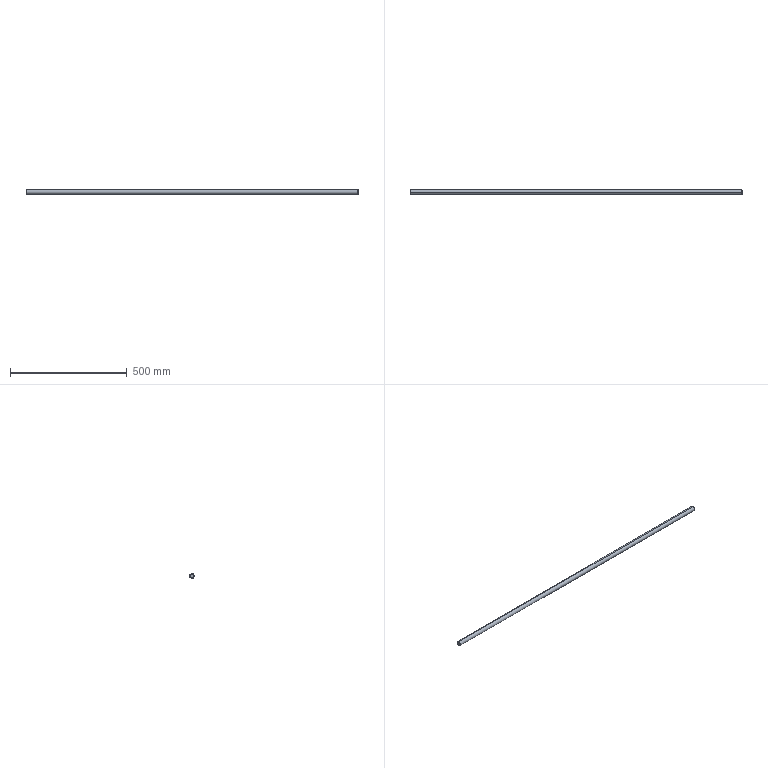Part | SolidWorks | features BaseBody 1 | 1 solid | 18 faces | box 1420 x 20 x 20 mm | volume 445152 mm3 | plane 8 | cone 6 | cylinder 4 | commonest cylinder face diameters 6 x2 20 x2
STEP:
#1=CARTESIAN_POINT('',(710.,0.,-9.));
#2=VERTEX_POINT('',#1);
#3=CARTESIAN_POINT('',(710.,8.485,-3.));
#4=VERTEX_POINT('',#3);
#5=CARTESIAN_POINT('',(710.,0.,0.));
#6=DIRECTION('',(1.,0.,0.));
#7=DIRECTION('',(0.,0.,-1.));
#8=AXIS2_PLACEMENT_3D('',#5,#6,#7);
#9=CIRCLE('',#8,9.);
#10=EDGE_CURVE('',#2,#4,#9,.T.);
#11=ORIENTED_EDGE('',*,*,#10,.F.);
#12=CARTESIAN_POINT('',(709.,0.,-10.));
#13=VERTEX_POINT('',#12);
#14=CARTESIAN_POINT('',(710.,0.,-9.));
#15=DIRECTION('',(-0.7071,0.,-0.7071));
#16=VECTOR('',#15,1000.);
#17=LINE('',#14,#16);
#18=EDGE_CURVE('',#2,#13,#17,.T.);
#19=ORIENTED_EDGE('',*,*,#18,.T.);
#20=CARTESIAN_POINT('',(709.,9.539,-3.));
#21=VERTEX_POINT('',#20);
#22=CARTESIAN_POINT('',(709.,0.,0.));
#23=DIRECTION('',(-1.,0.,0.));
#24=DIRECTION('',(0.,0.,-1.));
#25=AXIS2_PLACEMENT_3D('',#22,#23,#24);
#26=CIRCLE('',#25,10.);
#27=EDGE_CURVE('',#21,#13,#26,.T.);
#28=ORIENTED_EDGE('',*,*,#27,.F.);
#29=CARTESIAN_POINT('',(710.,8.485,-3.));
#30=CARTESIAN_POINT('',(709.668,8.838,-3.));
#31=CARTESIAN_POINT('',(709.334,9.189,-3.));
#32=CARTESIAN_POINT('',(709.,9.539,-3.));
#33=B_SPLINE_CURVE_WITH_KNOTS('',3,(#29,#30,#31,#32),.UNSPECIFIED.,.F.,.F.,(4,4),(0.005441,0.006894),.UNSPECIFIED.);
#34=EDGE_CURVE('',#4,#21,#33,.T.);
#35=ORIENTED_EDGE('',*,*,#34,.F.);
#36=EDGE_LOOP('',(#11,#19,#28,#35));
#37=FACE_OUTER_BOUND('',#36,.T.);
#38=CARTESIAN_POINT('',(710.,0.,0.));
#39=DIRECTION('',(-1.,0.,0.));
#40=DIRECTION('',(0.,0.,1.));
#41=AXIS2_PLACEMENT_3D('',#38,#39,#40);
#42=CONICAL_SURFACE('',#41,9.,0.7854);
#43=ADVANCED_FACE('',(#37),#42,.T.);
#44=ORIENTED_EDGE('',*,*,#18,.F.);
#45=CARTESIAN_POINT('',(710.,0.,9.));
#46=VERTEX_POINT('',#45);
#47=CARTESIAN_POINT('',(710.,0.,0.));
#48=DIRECTION('',(1.,0.,0.));
#49=DIRECTION('',(0.,0.,-1.));
#50=AXIS2_PLACEMENT_3D('',#47,#48,#49);
#51=CIRCLE('',#50,9.);
#52=EDGE_CURVE('',#46,#2,#51,.T.);
#53=ORIENTED_EDGE('',*,*,#52,.F.);
#54=CARTESIAN_POINT('',(709.,0.,10.));
#55=VERTEX_POINT('',#54);
#56=CARTESIAN_POINT('',(710.,0.,9.));
#57=DIRECTION('',(-0.7071,0.,0.7071));
#58=VECTOR('',#57,1000.);
#59=LINE('',#56,#58);
#60=EDGE_CURVE('',#46,#55,#59,.T.);
#61=ORIENTED_EDGE('',*,*,#60,.T.);
#62=CARTESIAN_POINT('',(709.,0.,0.));
#63=DIRECTION('',(-1.,0.,0.));
#64=DIRECTION('',(0.,0.,-1.));
#65=AXIS2_PLACEMENT_3D('',#62,#63,#64);
#66=CIRCLE('',#65,10.);
#67=EDGE_CURVE('',#13,#55,#66,.T.);
#68=ORIENTED_EDGE('',*,*,#67,.F.);
#69=EDGE_LOOP('',(#44,#53,#61,#68));
#70=FACE_OUTER_BOUND('',#69,.T.);
#71=CARTESIAN_POINT('',(710.,0.,0.));
#72=DIRECTION('',(-1.,0.,0.));
#73=DIRECTION('',(0.,0.,1.));
#74=AXIS2_PLACEMENT_3D('',#71,#72,#73);
#75=CONICAL_SURFACE('',#74,9.,0.7854);
#76=ADVANCED_FACE('',(#70),#75,.T.);
#77=CARTESIAN_POINT('',(-710.,0.,9.));
#78=VERTEX_POINT('',#77);
#79=CARTESIAN_POINT('',(-710.,8.485,3.));
#80=VERTEX_POINT('',#79);
#81=CARTESIAN_POINT('',(-710.,0.,0.));
#82=DIRECTION('',(-1.,0.,0.));
#83=DIRECTION('',(0.,0.,-1.));
#84=AXIS2_PLACEMENT_3D('',#81,#82,#83);
#85=CIRCLE('',#84,9.);
#86=EDGE_CURVE('',#78,#80,#85,.T.);
#87=ORIENTED_EDGE('',*,*,#86,.F.);
#88=CARTESIAN_POINT('',(-709.,0.,10.));
#89=VERTEX_POINT('',#88);
#90=CARTESIAN_POINT('',(-709.,0.,10.));
#91=DIRECTION('',(0.7071,0.,0.7071));
#92=VECTOR('',#91,1000.);
#93=LINE('',#90,#92);
#94=EDGE_CURVE('',#78,#89,#93,.T.);
#95=ORIENTED_EDGE('',*,*,#94,.T.);
#96=CARTESIAN_POINT('',(-709.,9.539,3.));
#97=VERTEX_POINT('',#96);
#98=CARTESIAN_POINT('',(-709.,0.,0.));
#99=DIRECTION('',(1.,0.,0.));
#100=DIRECTION('',(0.,0.,-1.));
#101=AXIS2_PLACEMENT_3D('',#98,#99,#100);
#102=CIRCLE('',#101,10.);
#103=EDGE_CURVE('',#97,#89,#102,.T.);
#104=ORIENTED_EDGE('',*,*,#103,.F.);
#105=CARTESIAN_POINT('',(-710.,8.485,3.));
#106=CARTESIAN_POINT('',(-709.668,8.838,3.));
#107=CARTESIAN_POINT('',(-709.334,9.189,3.));
#108=CARTESIAN_POINT('',(-709.,9.539,3.));
#109=B_SPLINE_CURVE_WITH_KNOTS('',3,(#105,#106,#107,#108),.UNSPECIFIED.,.F.,.F.,(4,4),(0.005441,0.006894),.UNSPECIFIED.);
#110=EDGE_CURVE('',#80,#97,#109,.T.);
#111=ORIENTED_EDGE('',*,*,#110,.F.);
#112=EDGE_LOOP('',(#87,#95,#104,#111));
#113=FACE_OUTER_BOUND('',#112,.T.);
#114=CARTESIAN_POINT('',(-709.,0.,0.));
#115=DIRECTION('',(1.,0.,0.));
#116=DIRECTION('',(0.,0.,-1.));
#117=AXIS2_PLACEMENT_3D('',#114,#115,#116);
#118=CONICAL_SURFACE('',#117,10.,0.7854);
#119=ADVANCED_FACE('',(#113),#118,.T.);
#120=ORIENTED_EDGE('',*,*,#94,.F.);
#121=CARTESIAN_POINT('',(-710.,0.,-9.));
#122=VERTEX_POINT('',#121);
#123=CARTESIAN_POINT('',(-710.,0.,0.));
#124=DIRECTION('',(-1.,0.,0.));
#125=DIRECTION('',(0.,0.,-1.));
#126=AXIS2_PLACEMENT_3D('',#123,#124,#125);
#127=CIRCLE('',#126,9.);
#128=EDGE_CURVE('',#122,#78,#127,.T.);
#129=ORIENTED_EDGE('',*,*,#128,.F.);
#130=CARTESIAN_POINT('',(-709.,0.,-10.));
#131=VERTEX_POINT('',#130);
#132=CARTESIAN_POINT('',(-709.,0.,-10.));
#133=DIRECTION('',(0.7071,0.,-0.7071));
#134=VECTOR('',#133,1000.);
#135=LINE('',#132,#134);
#136=EDGE_CURVE('',#122,#131,#135,.T.);
#137=ORIENTED_EDGE('',*,*,#136,.T.);
#138=CARTESIAN_POINT('',(-709.,0.,0.));
#139=DIRECTION('',(1.,0.,0.));
#140=DIRECTION('',(0.,0.,-1.));
#141=AXIS2_PLACEMENT_3D('',#138,#139,#140);
#142=CIRCLE('',#141,10.);
#143=EDGE_CURVE('',#89,#131,#142,.T.);
#144=ORIENTED_EDGE('',*,*,#143,.F.);
#145=EDGE_LOOP('',(#120,#129,#137,#144));
#146=FACE_OUTER_BOUND('',#145,.T.);
#147=CARTESIAN_POINT('',(-709.,0.,0.));
#148=DIRECTION('',(1.,0.,0.));
#149=DIRECTION('',(0.,0.,-1.));
#150=AXIS2_PLACEMENT_3D('',#147,#148,#149);
#151=CONICAL_SURFACE('',#150,10.,0.7854);
#152=ADVANCED_FACE('',(#146),#151,.T.);
#153=ORIENTED_EDGE('',*,*,#27,.T.);
#154=CARTESIAN_POINT('',(710.,0.,-10.));
#155=DIRECTION('',(-1.,0.,0.));
#156=VECTOR('',#155,1000.);
#157=LINE('',#154,#156);
#158=EDGE_CURVE('',#13,#131,#157,.T.);
#159=ORIENTED_EDGE('',*,*,#158,.T.);
#160=CARTESIAN_POINT('',(-709.,9.539,-3.));
#161=VERTEX_POINT('',#160);
#162=CARTESIAN_POINT('',(-709.,0.,0.));
#163=DIRECTION('',(1.,0.,0.));
#164=DIRECTION('',(0.,0.,-1.));
#165=AXIS2_PLACEMENT_3D('',#162,#163,#164);
#166=CIRCLE('',#165,10.);
#167=EDGE_CURVE('',#131,#161,#166,.T.);
#168=ORIENTED_EDGE('',*,*,#167,.T.);
#169=CARTESIAN_POINT('',(-690.,9.539,-3.));
#170=VERTEX_POINT('',#169);
#171=CARTESIAN_POINT('',(710.,9.539,-3.));
#172=DIRECTION('',(1.,0.,0.));
#173=VECTOR('',#172,1000.);
#174=LINE('',#171,#173);
#175=EDGE_CURVE('',#161,#170,#174,.T.);
#176=ORIENTED_EDGE('',*,*,#175,.T.);
#177=CARTESIAN_POINT('',(-690.,9.539,3.));
#178=VERTEX_POINT('',#177);
#179=CARTESIAN_POINT('',(-690.,9.539,-3.));
#180=CARTESIAN_POINT('',(-689.804,9.539,-3.));
#181=CARTESIAN_POINT('',(-689.607,9.546,-2.981));
#182=CARTESIAN_POINT('',(-689.217,9.569,-2.903));
#183=CARTESIAN_POINT('',(-689.03,9.587,-2.845));
#184=CARTESIAN_POINT('',(-688.668,9.63,-2.695));
#185=CARTESIAN_POINT('',(-688.492,9.656,-2.601));
#186=CARTESIAN_POINT('',(-688.168,9.712,-2.384));
#187=CARTESIAN_POINT('',(-688.018,9.742,-2.26));
#188=CARTESIAN_POINT('',(-687.741,9.802,-1.984));
#189=CARTESIAN_POINT('',(-687.616,9.832,-1.831));
#190=CARTESIAN_POINT('',(-687.399,9.887,-1.508));
#191=CARTESIAN_POINT('',(-687.306,9.912,-1.335));
#192=CARTESIAN_POINT('',(-687.154,9.955,-0.9694));
#193=CARTESIAN_POINT('',(-687.097,9.971,-0.7818));
#194=CARTESIAN_POINT('',(-687.02,9.994,-0.3973));
#195=CARTESIAN_POINT('',(-687.,10.,-0.1979));
#196=CARTESIAN_POINT('',(-687.,10.,0.1975));
#197=CARTESIAN_POINT('',(-687.019,9.994,0.393));
#198=CARTESIAN_POINT('',(-687.096,9.971,0.7797));
#199=CARTESIAN_POINT('',(-687.155,9.954,0.971));
#200=CARTESIAN_POINT('',(-687.38,9.892,1.513));
#201=CARTESIAN_POINT('',(-687.603,9.832,1.846));
#202=CARTESIAN_POINT('',(-688.016,9.743,2.258));
#203=CARTESIAN_POINT('',(-688.169,9.712,2.384));
#204=CARTESIAN_POINT('',(-688.494,9.656,2.602));
#205=CARTESIAN_POINT('',(-688.665,9.631,2.694));
#206=CARTESIAN_POINT('',(-689.027,9.587,2.845));
#207=CARTESIAN_POINT('',(-689.219,9.569,2.903));
#208=CARTESIAN_POINT('',(-689.604,9.546,2.98));
#209=CARTESIAN_POINT('',(-689.801,9.539,3.));
#210=CARTESIAN_POINT('',(-690.,9.539,3.));
#211=B_SPLINE_CURVE_WITH_KNOTS('',3,(#179,#180,#181,#182,#183,#184,#185,#186,#187,#188,#189,#190,#191,#192,#193,#194,#195,#196,#197,#198,#199,#200,#201,#202,#203,#204,#205,#206,#207,#208,#209,#210),.UNSPECIFIED.,.F.,.F.,(4,2,2,2,2,2,2,2,2,2,2,2,2,2,2,4),(0.009434,0.01002,0.01061,0.0112,0.01179,0.01238,0.01297,0.01356,0.01415,0.01474,0.01533,0.01651,0.0171,0.01769,0.01828,0.01887),.UNSPECIFIED.);
#212=EDGE_CURVE('',#170,#178,#211,.T.);
#213=ORIENTED_EDGE('',*,*,#212,.T.);
#214=CARTESIAN_POINT('',(710.,9.539,3.));
#215=DIRECTION('',(-1.,0.,0.));
#216=VECTOR('',#215,1000.);
#217=LINE('',#214,#216);
#218=EDGE_CURVE('',#178,#97,#217,.T.);
#219=ORIENTED_EDGE('',*,*,#218,.T.);
#220=ORIENTED_EDGE('',*,*,#103,.T.);
#221=CARTESIAN_POINT('',(710.,0.,10.));
#222=DIRECTION('',(-1.,0.,0.));
#223=VECTOR('',#222,1000.);
#224=LINE('',#221,#223);
#225=EDGE_CURVE('',#55,#89,#224,.T.);
#226=ORIENTED_EDGE('',*,*,#225,.F.);
#227=CARTESIAN_POINT('',(709.,9.539,3.));
#228=VERTEX_POINT('',#227);
#229=CARTESIAN_POINT('',(709.,0.,0.));
#230=DIRECTION('',(-1.,0.,0.));
#231=DIRECTION('',(0.,0.,-1.));
#232=AXIS2_PLACEMENT_3D('',#229,#230,#231);
#233=CIRCLE('',#232,10.);
#234=EDGE_CURVE('',#55,#228,#233,.T.);
#235=ORIENTED_EDGE('',*,*,#234,.T.);
#236=CARTESIAN_POINT('',(690.,9.539,3.));
#237=VERTEX_POINT('',#236);
#238=CARTESIAN_POINT('',(710.,9.539,3.));
#239=DIRECTION('',(-1.,0.,0.));
#240=VECTOR('',#239,1000.);
#241=LINE('',#238,#240);
#242=EDGE_CURVE('',#228,#237,#241,.T.);
#243=ORIENTED_EDGE('',*,*,#242,.T.);
#244=CARTESIAN_POINT('',(690.,9.539,-3.));
#245=VERTEX_POINT('',#244);
#246=CARTESIAN_POINT('',(690.,9.539,3.));
#247=CARTESIAN_POINT('',(689.801,9.539,3.));
#248=CARTESIAN_POINT('',(689.605,9.546,2.98));
#249=CARTESIAN_POINT('',(689.22,9.569,2.903));
#250=CARTESIAN_POINT('',(689.029,9.587,2.845));
#251=CARTESIAN_POINT('',(688.666,9.631,2.694));
#252=CARTESIAN_POINT('',(688.494,9.656,2.602));
#253=CARTESIAN_POINT('',(688.169,9.712,2.385));
#254=CARTESIAN_POINT('',(688.016,9.743,2.259));
#255=CARTESIAN_POINT('',(687.604,9.832,1.847));
#256=CARTESIAN_POINT('',(687.381,9.891,1.514));
#257=CARTESIAN_POINT('',(687.156,9.954,0.9732));
#258=CARTESIAN_POINT('',(687.097,9.971,0.783));
#259=CARTESIAN_POINT('',(687.02,9.994,0.3953));
#260=CARTESIAN_POINT('',(687.,10.,0.1999));
#261=CARTESIAN_POINT('',(687.,10.,-0.194));
#262=CARTESIAN_POINT('',(687.019,9.994,-0.394));
#263=CARTESIAN_POINT('',(687.096,9.971,-0.7797));
#264=CARTESIAN_POINT('',(687.153,9.955,-0.9673));
#265=CARTESIAN_POINT('',(687.305,9.913,-1.332));
#266=CARTESIAN_POINT('',(687.398,9.887,-1.506));
#267=CARTESIAN_POINT('',(687.614,9.833,-1.83));
#268=CARTESIAN_POINT('',(687.74,9.803,-1.982));
#269=CARTESIAN_POINT('',(688.016,9.743,-2.259));
#270=CARTESIAN_POINT('',(688.167,9.713,-2.383));
#271=CARTESIAN_POINT('',(688.49,9.657,-2.6));
#272=CARTESIAN_POINT('',(688.666,9.631,-2.694));
#273=CARTESIAN_POINT('',(689.027,9.587,-2.845));
#274=CARTESIAN_POINT('',(689.214,9.57,-2.902));
#275=CARTESIAN_POINT('',(689.601,9.546,-2.98));
#276=CARTESIAN_POINT('',(689.801,9.539,-3.));
#277=CARTESIAN_POINT('',(690.,9.539,-3.));
#278=B_SPLINE_CURVE_WITH_KNOTS('',3,(#246,#247,#248,#249,#250,#251,#252,#253,#254,#255,#256,#257,#258,#259,#260,#261,#262,#263,#264,#265,#266,#267,#268,#269,#270,#271,#272,#273,#274,#275,#276,#277),.UNSPECIFIED.,.F.,.F.,(4,2,2,2,2,2,2,2,2,2,2,2,2,2,2,4),(0.,0.0005894,0.001179,0.001768,0.002358,0.003536,0.004126,0.004715,0.005305,0.005894,0.006484,0.007073,0.007662,0.008252,0.008841,0.009431),.UNSPECIFIED.);
#279=EDGE_CURVE('',#237,#245,#278,.T.);
#280=ORIENTED_EDGE('',*,*,#279,.T.);
#281=CARTESIAN_POINT('',(710.,9.539,-3.));
#282=DIRECTION('',(1.,0.,0.));
#283=VECTOR('',#282,1000.);
#284=LINE('',#281,#283);
#285=EDGE_CURVE('',#245,#21,#284,.T.);
#286=ORIENTED_EDGE('',*,*,#285,.T.);
#287=EDGE_LOOP('',(#153,#159,#168,#176,#213,#219,#220,#226,#235,#243,#280,#286));
#288=FACE_OUTER_BOUND('',#287,.T.);
#289=CARTESIAN_POINT('',(710.,0.,0.));
#290=DIRECTION('',(-1.,0.,0.));
#291=DIRECTION('',(0.,0.,1.));
#292=AXIS2_PLACEMENT_3D('',#289,#290,#291);
#293=CYLINDRICAL_SURFACE('',#292,10.);
#294=ADVANCED_FACE('',(#288),#293,.T.);
#295=ORIENTED_EDGE('',*,*,#158,.F.);
#296=ORIENTED_EDGE('',*,*,#67,.T.);
#297=ORIENTED_EDGE('',*,*,#225,.T.);
#298=ORIENTED_EDGE('',*,*,#143,.T.);
#299=EDGE_LOOP('',(#295,#296,#297,#298));
#300=FACE_OUTER_BOUND('',#299,.T.);
#301=CARTESIAN_POINT('',(710.,0.,0.));
#302=DIRECTION('',(-1.,0.,0.));
#303=DIRECTION('',(0.,0.,1.));
#304=AXIS2_PLACEMENT_3D('',#301,#302,#303);
#305=CYLINDRICAL_SURFACE('',#304,10.);
#306=ADVANCED_FACE('',(#300),#305,.T.);
#307=CARTESIAN_POINT('',(710.,6.5,3.));
#308=VERTEX_POINT('',#307);
#309=CARTESIAN_POINT('',(710.,8.485,3.));
#310=VERTEX_POINT('',#309);
#311=CARTESIAN_POINT('',(710.,6.5,3.));
#312=DIRECTION('',(0.,1.,0.));
#313=VECTOR('',#312,1000.);
#314=LINE('',#311,#313);
#315=EDGE_CURVE('',#308,#310,#314,.T.);
#316=ORIENTED_EDGE('',*,*,#315,.T.);
#317=CARTESIAN_POINT('',(710.,0.,0.));
#318=DIRECTION('',(1.,0.,0.));
#319=DIRECTION('',(0.,0.,-1.));
#320=AXIS2_PLACEMENT_3D('',#317,#318,#319);
#321=CIRCLE('',#320,9.);
#322=EDGE_CURVE('',#310,#46,#321,.T.);
#323=ORIENTED_EDGE('',*,*,#322,.T.);
#324=ORIENTED_EDGE('',*,*,#52,.T.);
#325=ORIENTED_EDGE('',*,*,#10,.T.);
#326=CARTESIAN_POINT('',(710.,6.5,-3.));
#327=VERTEX_POINT('',#326);
#328=CARTESIAN_POINT('',(710.,6.5,-3.));
#329=DIRECTION('',(0.,1.,0.));
#330=VECTOR('',#329,1000.);
#331=LINE('',#328,#330);
#332=EDGE_CURVE('',#327,#4,#331,.T.);
#333=ORIENTED_EDGE('',*,*,#332,.F.);
#334=CARTESIAN_POINT('',(710.,6.5,0.));
#335=DIRECTION('',(0.,0.,-1.));
#336=VECTOR('',#335,1000.);
#337=LINE('',#334,#336);
#338=EDGE_CURVE('',#308,#327,#337,.T.);
#339=ORIENTED_EDGE('',*,*,#338,.F.);
#340=EDGE_LOOP('',(#316,#323,#324,#325,#333,#339));
#341=FACE_OUTER_BOUND('',#340,.T.);
#342=CARTESIAN_POINT('',(710.,0.,0.));
#343=DIRECTION('',(1.,0.,0.));
#344=DIRECTION('',(0.,0.,-1.));
#345=AXIS2_PLACEMENT_3D('',#342,#343,#344);
#346=PLANE('',#345);
#347=ADVANCED_FACE('',(#341),#346,.T.);
#348=CARTESIAN_POINT('',(-710.,6.5,-3.));
#349=VERTEX_POINT('',#348);
#350=CARTESIAN_POINT('',(-710.,6.5,3.));
#351=VERTEX_POINT('',#350);
#352=CARTESIAN_POINT('',(-710.,6.5,0.));
#353=DIRECTION('',(0.,0.,1.));
#354=VECTOR('',#353,1000.);
#355=LINE('',#352,#354);
#356=EDGE_CURVE('',#349,#351,#355,.T.);
#357=ORIENTED_EDGE('',*,*,#356,.F.);
#358=CARTESIAN_POINT('',(-710.,8.485,-3.));
#359=VERTEX_POINT('',#358);
#360=CARTESIAN_POINT('',(-710.,6.5,-3.));
#361=DIRECTION('',(0.,1.,0.));
#362=VECTOR('',#361,1000.);
#363=LINE('',#360,#362);
#364=EDGE_CURVE('',#349,#359,#363,.T.);
#365=ORIENTED_EDGE('',*,*,#364,.T.);
#366=CARTESIAN_POINT('',(-710.,0.,0.));
#367=DIRECTION('',(-1.,0.,0.));
#368=DIRECTION('',(0.,0.,-1.));
#369=AXIS2_PLACEMENT_3D('',#366,#367,#368);
#370=CIRCLE('',#369,9.);
#371=EDGE_CURVE('',#359,#122,#370,.T.);
#372=ORIENTED_EDGE('',*,*,#371,.T.);
#373=ORIENTED_EDGE('',*,*,#128,.T.);
#374=ORIENTED_EDGE('',*,*,#86,.T.);
#375=CARTESIAN_POINT('',(-710.,6.5,3.));
#376=DIRECTION('',(0.,1.,0.));
#377=VECTOR('',#376,1000.);
#378=LINE('',#375,#377);
#379=EDGE_CURVE('',#351,#80,#378,.T.);
#380=ORIENTED_EDGE('',*,*,#379,.F.);
#381=EDGE_LOOP('',(#357,#365,#372,#373,#374,#380));
#382=FACE_OUTER_BOUND('',#381,.T.);
#383=CARTESIAN_POINT('',(-710.,0.,0.));
#384=DIRECTION('',(1.,0.,0.));
#385=DIRECTION('',(0.,0.,-1.));
#386=AXIS2_PLACEMENT_3D('',#383,#384,#385);
#387=PLANE('',#386);
#388=ADVANCED_FACE('',(#382),#387,.F.);
#389=ORIENTED_EDGE('',*,*,#136,.F.);
#390=ORIENTED_EDGE('',*,*,#371,.F.);
#391=CARTESIAN_POINT('',(-709.,9.539,-3.));
#392=CARTESIAN_POINT('',(-709.334,9.189,-3.));
#393=CARTESIAN_POINT('',(-709.668,8.838,-3.));
#394=CARTESIAN_POINT('',(-710.,8.485,-3.));
#395=B_SPLINE_CURVE_WITH_KNOTS('',3,(#391,#392,#393,#394),.UNSPECIFIED.,.F.,.F.,(4,4),(0.005238,0.006691),.UNSPECIFIED.);
#396=EDGE_CURVE('',#161,#359,#395,.T.);
#397=ORIENTED_EDGE('',*,*,#396,.F.);
#398=ORIENTED_EDGE('',*,*,#167,.F.);
#399=EDGE_LOOP('',(#389,#390,#397,#398));
#400=FACE_OUTER_BOUND('',#399,.T.);
#401=CARTESIAN_POINT('',(-709.,0.,0.));
#402=DIRECTION('',(1.,0.,0.));
#403=DIRECTION('',(0.,0.,-1.));
#404=AXIS2_PLACEMENT_3D('',#401,#402,#403);
#405=CONICAL_SURFACE('',#404,10.,0.7854);
#406=ADVANCED_FACE('',(#400),#405,.T.);
#407=ORIENTED_EDGE('',*,*,#60,.F.);
#408=ORIENTED_EDGE('',*,*,#322,.F.);
#409=CARTESIAN_POINT('',(709.,9.539,3.));
#410=CARTESIAN_POINT('',(709.334,9.189,3.));
#411=CARTESIAN_POINT('',(709.668,8.838,3.));
#412=CARTESIAN_POINT('',(710.,8.485,3.));
#413=B_SPLINE_CURVE_WITH_KNOTS('',3,(#409,#410,#411,#412),.UNSPECIFIED.,.F.,.F.,(4,4),(0.005238,0.006691),.UNSPECIFIED.);
#414=EDGE_CURVE('',#228,#310,#413,.T.);
#415=ORIENTED_EDGE('',*,*,#414,.F.);
#416=ORIENTED_EDGE('',*,*,#234,.F.);
#417=EDGE_LOOP('',(#407,#408,#415,#416));
#418=FACE_OUTER_BOUND('',#417,.T.);
#419=CARTESIAN_POINT('',(710.,0.,0.));
#420=DIRECTION('',(-1.,0.,0.));
#421=DIRECTION('',(0.,0.,1.));
#422=AXIS2_PLACEMENT_3D('',#419,#420,#421);
#423=CONICAL_SURFACE('',#422,9.,0.7854);
#424=ADVANCED_FACE('',(#418),#423,.T.);
#425=CARTESIAN_POINT('',(690.,6.5,3.));
#426=VERTEX_POINT('',#425);
#427=CARTESIAN_POINT('',(690.,6.5,3.));
#428=DIRECTION('',(0.,1.,0.));
#429=VECTOR('',#428,1000.);
#430=LINE('',#427,#429);
#431=EDGE_CURVE('',#426,#237,#430,.T.);
#432=ORIENTED_EDGE('',*,*,#431,.F.);
#433=CARTESIAN_POINT('',(690.,6.5,-3.));
#434=VERTEX_POINT('',#433);
#435=CARTESIAN_POINT('',(690.,6.5,0.));
#436=DIRECTION('',(0.,1.,0.));
#437=DIRECTION('',(0.,0.,-1.));
#438=AXIS2_PLACEMENT_3D('',#435,#436,#437);
#439=CIRCLE('',#438,3.);
#440=EDGE_CURVE('',#434,#426,#439,.T.);
#441=ORIENTED_EDGE('',*,*,#440,.F.);
#442=CARTESIAN_POINT('',(690.,6.5,-3.));
#443=DIRECTION('',(0.,1.,0.));
#444=VECTOR('',#443,1000.);
#445=LINE('',#442,#444);
#446=EDGE_CURVE('',#434,#245,#445,.T.);
#447=ORIENTED_EDGE('',*,*,#446,.T.);
#448=ORIENTED_EDGE('',*,*,#279,.F.);
#449=EDGE_LOOP('',(#432,#441,#447,#448));
#450=FACE_OUTER_BOUND('',#449,.T.);
#451=CARTESIAN_POINT('',(690.,6.5,0.));
#452=DIRECTION('',(0.,1.,0.));
#453=DIRECTION('',(0.,0.,1.));
#454=AXIS2_PLACEMENT_3D('',#451,#452,#453);
#455=CYLINDRICAL_SURFACE('',#454,3.);
#456=ADVANCED_FACE('',(#450),#455,.F.);
#457=ORIENTED_EDGE('',*,*,#414,.T.);
#458=ORIENTED_EDGE('',*,*,#315,.F.);
#459=CARTESIAN_POINT('',(710.,6.5,3.));
#460=DIRECTION('',(1.,0.,0.));
#461=VECTOR('',#460,1000.);
#462=LINE('',#459,#461);
#463=EDGE_CURVE('',#426,#308,#462,.T.);
#464=ORIENTED_EDGE('',*,*,#463,.F.);
#465=ORIENTED_EDGE('',*,*,#431,.T.);
#466=ORIENTED_EDGE('',*,*,#242,.F.);
#467=EDGE_LOOP('',(#457,#458,#464,#465,#466));
#468=FACE_OUTER_BOUND('',#467,.T.);
#469=CARTESIAN_POINT('',(710.,6.5,3.));
#470=DIRECTION('',(0.,0.,1.));
#471=DIRECTION('',(1.,0.,0.));
#472=AXIS2_PLACEMENT_3D('',#469,#470,#471);
#473=PLANE('',#472);
#474=ADVANCED_FACE('',(#468),#473,.F.);
#475=ORIENTED_EDGE('',*,*,#446,.F.);
#476=CARTESIAN_POINT('',(710.,6.5,-3.));
#477=DIRECTION('',(-1.,0.,0.));
#478=VECTOR('',#477,1000.);
#479=LINE('',#476,#478);
#480=EDGE_CURVE('',#327,#434,#479,.T.);
#481=ORIENTED_EDGE('',*,*,#480,.F.);
#482=ORIENTED_EDGE('',*,*,#332,.T.);
#483=ORIENTED_EDGE('',*,*,#34,.T.);
#484=ORIENTED_EDGE('',*,*,#285,.F.);
#485=EDGE_LOOP('',(#475,#481,#482,#483,#484));
#486=FACE_OUTER_BOUND('',#485,.T.);
#487=CARTESIAN_POINT('',(710.,6.5,-3.));
#488=DIRECTION('',(0.,0.,-1.));
#489=DIRECTION('',(-1.,0.,0.));
#490=AXIS2_PLACEMENT_3D('',#487,#488,#489);
#491=PLANE('',#490);
#492=ADVANCED_FACE('',(#486),#491,.F.);
#493=ORIENTED_EDGE('',*,*,#338,.T.);
#494=ORIENTED_EDGE('',*,*,#480,.T.);
#495=ORIENTED_EDGE('',*,*,#440,.T.);
#496=ORIENTED_EDGE('',*,*,#463,.T.);
#497=EDGE_LOOP('',(#493,#494,#495,#496));
#498=FACE_OUTER_BOUND('',#497,.T.);
#499=CARTESIAN_POINT('',(710.,6.5,0.));
#500=DIRECTION('',(0.,-1.,0.));
#501=DIRECTION('',(0.,0.,-1.));
#502=AXIS2_PLACEMENT_3D('',#499,#500,#501);
#503=PLANE('',#502);
#504=ADVANCED_FACE('',(#498),#503,.F.);
#505=CARTESIAN_POINT('',(-690.,6.5,-3.));
#506=VERTEX_POINT('',#505);
#507=CARTESIAN_POINT('',(-690.,6.5,-3.));
#508=DIRECTION('',(0.,1.,0.));
#509=VECTOR('',#508,1000.);
#510=LINE('',#507,#509);
#511=EDGE_CURVE('',#506,#170,#510,.T.);
#512=ORIENTED_EDGE('',*,*,#511,.F.);
#513=CARTESIAN_POINT('',(-690.,6.5,3.));
#514=VERTEX_POINT('',#513);
#515=CARTESIAN_POINT('',(-690.,6.5,0.));
#516=DIRECTION('',(0.,1.,0.));
#517=DIRECTION('',(0.,0.,1.));
#518=AXIS2_PLACEMENT_3D('',#515,#516,#517);
#519=CIRCLE('',#518,3.);
#520=EDGE_CURVE('',#514,#506,#519,.T.);
#521=ORIENTED_EDGE('',*,*,#520,.F.);
#522=CARTESIAN_POINT('',(-690.,6.5,3.));
#523=DIRECTION('',(0.,1.,0.));
#524=VECTOR('',#523,1000.);
#525=LINE('',#522,#524);
#526=EDGE_CURVE('',#514,#178,#525,.T.);
#527=ORIENTED_EDGE('',*,*,#526,.T.);
#528=ORIENTED_EDGE('',*,*,#212,.F.);
#529=EDGE_LOOP('',(#512,#521,#527,#528));
#530=FACE_OUTER_BOUND('',#529,.T.);
#531=CARTESIAN_POINT('',(-690.,6.5,0.));
#532=DIRECTION('',(0.,1.,0.));
#533=DIRECTION('',(0.,0.,1.));
#534=AXIS2_PLACEMENT_3D('',#531,#532,#533);
#535=CYLINDRICAL_SURFACE('',#534,3.);
#536=ADVANCED_FACE('',(#530),#535,.F.);
#537=ORIENTED_EDGE('',*,*,#356,.T.);
#538=CARTESIAN_POINT('',(-710.,6.5,3.));
#539=DIRECTION('',(1.,0.,0.));
#540=VECTOR('',#539,1000.);
#541=LINE('',#538,#540);
#542=EDGE_CURVE('',#351,#514,#541,.T.);
#543=ORIENTED_EDGE('',*,*,#542,.T.);
#544=ORIENTED_EDGE('',*,*,#520,.T.);
#545=CARTESIAN_POINT('',(-710.,6.5,-3.));
#546=DIRECTION('',(-1.,0.,0.));
#547=VECTOR('',#546,1000.);
#548=LINE('',#545,#547);
#549=EDGE_CURVE('',#506,#349,#548,.T.);
#550=ORIENTED_EDGE('',*,*,#549,.T.);
#551=EDGE_LOOP('',(#537,#543,#544,#550));
#552=FACE_OUTER_BOUND('',#551,.T.);
#553=CARTESIAN_POINT('',(-710.,6.5,0.));
#554=DIRECTION('',(0.,1.,0.));
#555=DIRECTION('',(0.,0.,1.));
#556=AXIS2_PLACEMENT_3D('',#553,#554,#555);
#557=PLANE('',#556);
#558=ADVANCED_FACE('',(#552),#557,.T.);
#559=ORIENTED_EDGE('',*,*,#396,.T.);
#560=ORIENTED_EDGE('',*,*,#364,.F.);
#561=ORIENTED_EDGE('',*,*,#549,.F.);
#562=ORIENTED_EDGE('',*,*,#511,.T.);
#563=ORIENTED_EDGE('',*,*,#175,.F.);
#564=EDGE_LOOP('',(#559,#560,#561,#562,#563));
#565=FACE_OUTER_BOUND('',#564,.T.);
#566=CARTESIAN_POINT('',(-710.,6.5,-3.));
#567=DIRECTION('',(0.,0.,-1.));
#568=DIRECTION('',(-1.,0.,0.));
#569=AXIS2_PLACEMENT_3D('',#566,#567,#568);
#570=PLANE('',#569);
#571=ADVANCED_FACE('',(#565),#570,.F.);
#572=ORIENTED_EDGE('',*,*,#526,.F.);
#573=ORIENTED_EDGE('',*,*,#542,.F.);
#574=ORIENTED_EDGE('',*,*,#379,.T.);
#575=ORIENTED_EDGE('',*,*,#110,.T.);
#576=ORIENTED_EDGE('',*,*,#218,.F.);
#577=EDGE_LOOP('',(#572,#573,#574,#575,#576));
#578=FACE_OUTER_BOUND('',#577,.T.);
#579=CARTESIAN_POINT('',(-710.,6.5,3.));
#580=DIRECTION('',(0.,0.,1.));
#581=DIRECTION('',(1.,0.,0.));
#582=AXIS2_PLACEMENT_3D('',#579,#580,#581);
#583=PLANE('',#582);
#584=ADVANCED_FACE('',(#578),#583,.F.);
#585=CLOSED_SHELL('',(#43,#76,#119,#152,#294,#306,#347,#388,#406,#424,#456,#474,#492,#504,#536,#558,#571,#584));
#586=MANIFOLD_SOLID_BREP('',#585);
#587=CARTESIAN_POINT('',(0.,0.,0.));
#588=DIRECTION('',(0.,0.,1.));
#589=DIRECTION('',(1.,0.,0.));
#590=AXIS2_PLACEMENT_3D('',#587,#588,#589);
#591=(LENGTH_UNIT()NAMED_UNIT(*)SI_UNIT(.MILLI.,.METRE.));
#592=UNCERTAINTY_MEASURE_WITH_UNIT(LENGTH_MEASURE(0.00001),#591,'','');
#593=(NAMED_UNIT(*)PLANE_ANGLE_UNIT()SI_UNIT($,.RADIAN.));
#594=(NAMED_UNIT(*)SI_UNIT($,.STERADIAN.)SOLID_ANGLE_UNIT());
#595=(GEOMETRIC_REPRESENTATION_CONTEXT(3)GLOBAL_UNCERTAINTY_ASSIGNED_CONTEXT((#592))GLOBAL_UNIT_ASSIGNED_CONTEXT((#591,#593,#594))REPRESENTATION_CONTEXT('',''));
#596=ADVANCED_BREP_SHAPE_REPRESENTATION('',(#586,#590),#595);